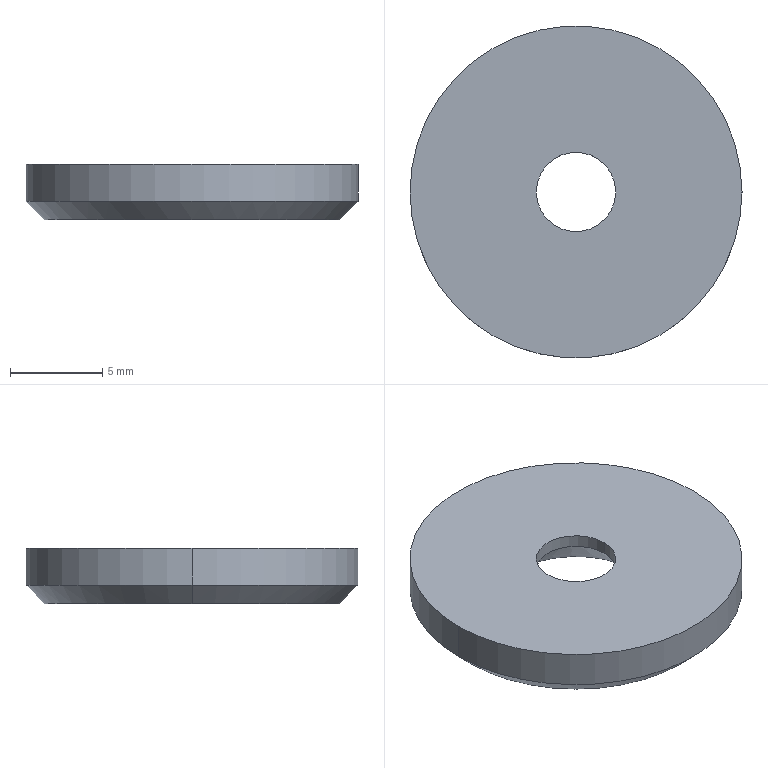Part | STEP file | 14 | 1 solid | 10 faces | box 18 x 18 x 3 mm | volume 644.142 mm3 | cylinder 4 | cone 4 | plane 2 | commonest cylinder face diameters 4.3 x2 18 x2
STEP:
#1=CARTESIAN_POINT('',(0.,0.,0.));
#2=DIRECTION('',(0.,0.,1.));
#3=DIRECTION('',(1.,0.,0.));
#4=AXIS2_PLACEMENT_3D('',#1,#2,#3);
#5=CARTESIAN_POINT('',(-101.,-48.,25.));
#6=VERTEX_POINT('',#5);
#7=CARTESIAN_POINT('',(-119.,-48.,25.));
#8=VERTEX_POINT('',#7);
#9=CARTESIAN_POINT('',(-110.,-48.,25.));
#10=DIRECTION('',(0.,0.,1.));
#11=DIRECTION('',(-1.,0.,0.));
#12=AXIS2_PLACEMENT_3D('',#9,#10,#11);
#13=CIRCLE('',#12,9.);
#14=CARTESIAN_POINT('',(-110.,-48.,23.5));
#15=DIRECTION('',(0.,0.,-1.));
#16=DIRECTION('',(-1.,0.,0.));
#17=AXIS2_PLACEMENT_3D('',#14,#15,#16);
#18=CYLINDRICAL_SURFACE('',#17,9.);
#19=CARTESIAN_POINT('',(6.283,-1.5));
#20=DIRECTION('',(-1.,0.));
#21=VECTOR('',#20,1.);
#22=LINE('',#19,#21);
#23=(GEOMETRIC_REPRESENTATION_CONTEXT(2)PARAMETRIC_REPRESENTATION_CONTEXT()REPRESENTATION_CONTEXT('',''));
#24=DEFINITIONAL_REPRESENTATION('',(#22),#23);
#25=PCURVE('',#18,#24);
#26=CARTESIAN_POINT('',(-105.5,-48.,25.));
#27=DIRECTION('',(0.,0.,1.));
#28=DIRECTION('',(1.,0.,0.));
#29=AXIS2_PLACEMENT_3D('',#26,#27,#28);
#30=PLANE('',#29);
#31=CARTESIAN_POINT('',(-4.5,0.));
#32=DIRECTION('',(-1.,0.));
#33=AXIS2_PLACEMENT_2D('',#31,#32);
#34=CIRCLE('',#33,9.);
#35=(GEOMETRIC_REPRESENTATION_CONTEXT(2)PARAMETRIC_REPRESENTATION_CONTEXT()REPRESENTATION_CONTEXT('',''));
#36=DEFINITIONAL_REPRESENTATION('',(#34),#35);
#37=PCURVE('',#30,#36);
#38=SURFACE_CURVE('',#13,(#25,#37),.PCURVE_S1.);
#39=EDGE_CURVE('',#6,#8,#38,.T.);
#40=ORIENTED_EDGE('',*,*,#39,.F.);
#41=CARTESIAN_POINT('',(-101.,-48.,23.));
#42=VERTEX_POINT('',#41);
#43=CARTESIAN_POINT('',(-101.,-48.,23.5));
#44=DIRECTION('',(0.,0.,-1.));
#45=VECTOR('',#44,1.);
#46=LINE('',#43,#45);
#47=CARTESIAN_POINT('',(3.142,0.));
#48=DIRECTION('',(0.,1.));
#49=VECTOR('',#48,1.);
#50=LINE('',#47,#49);
#51=(GEOMETRIC_REPRESENTATION_CONTEXT(2)PARAMETRIC_REPRESENTATION_CONTEXT()REPRESENTATION_CONTEXT('',''));
#52=DEFINITIONAL_REPRESENTATION('',(#50),#51);
#53=PCURVE('',#18,#52);
#54=CARTESIAN_POINT('',(-110.,-48.,23.5));
#55=DIRECTION('',(0.,0.,-1.));
#56=DIRECTION('',(-1.,0.,0.));
#57=AXIS2_PLACEMENT_3D('',#54,#55,#56);
#58=CYLINDRICAL_SURFACE('',#57,9.);
#59=CARTESIAN_POINT('',(3.142,0.));
#60=DIRECTION('',(0.,1.));
#61=VECTOR('',#60,1.);
#62=LINE('',#59,#61);
#63=(GEOMETRIC_REPRESENTATION_CONTEXT(2)PARAMETRIC_REPRESENTATION_CONTEXT()REPRESENTATION_CONTEXT('',''));
#64=DEFINITIONAL_REPRESENTATION('',(#62),#63);
#65=PCURVE('',#58,#64);
#66=SURFACE_CURVE('',#46,(#53,#65),.PCURVE_S1.);
#67=EDGE_CURVE('',#6,#42,#66,.T.);
#68=ORIENTED_EDGE('',*,*,#67,.T.);
#69=CARTESIAN_POINT('',(-119.,-48.,23.));
#70=VERTEX_POINT('',#69);
#71=CARTESIAN_POINT('',(-110.,-48.,23.));
#72=DIRECTION('',(0.,0.,1.));
#73=DIRECTION('',(-1.,0.,0.));
#74=AXIS2_PLACEMENT_3D('',#71,#72,#73);
#75=CIRCLE('',#74,9.);
#76=CARTESIAN_POINT('',(6.283,0.5));
#77=DIRECTION('',(-1.,0.));
#78=VECTOR('',#77,1.);
#79=LINE('',#76,#78);
#80=(GEOMETRIC_REPRESENTATION_CONTEXT(2)PARAMETRIC_REPRESENTATION_CONTEXT()REPRESENTATION_CONTEXT('',''));
#81=DEFINITIONAL_REPRESENTATION('',(#79),#80);
#82=PCURVE('',#18,#81);
#83=CARTESIAN_POINT('',(-110.,-48.,23.));
#84=DIRECTION('',(0.,0.,1.));
#85=DIRECTION('',(1.,0.,0.));
#86=AXIS2_PLACEMENT_3D('',#83,#84,#85);
#87=CONICAL_SURFACE('',#86,9.,0.7854);
#88=CARTESIAN_POINT('',(-3.142,0.));
#89=DIRECTION('',(1.,0.));
#90=VECTOR('',#89,1.);
#91=LINE('',#88,#90);
#92=(GEOMETRIC_REPRESENTATION_CONTEXT(2)PARAMETRIC_REPRESENTATION_CONTEXT()REPRESENTATION_CONTEXT('',''));
#93=DEFINITIONAL_REPRESENTATION('',(#91),#92);
#94=PCURVE('',#87,#93);
#95=SURFACE_CURVE('',#75,(#82,#94),.PCURVE_S1.);
#96=EDGE_CURVE('',#42,#70,#95,.T.);
#97=ORIENTED_EDGE('',*,*,#96,.T.);
#98=CARTESIAN_POINT('',(-119.,-48.,23.5));
#99=DIRECTION('',(0.,0.,-1.));
#100=VECTOR('',#99,1.);
#101=LINE('',#98,#100);
#102=CARTESIAN_POINT('',(0.,0.));
#103=DIRECTION('',(0.,1.));
#104=VECTOR('',#103,1.);
#105=LINE('',#102,#104);
#106=(GEOMETRIC_REPRESENTATION_CONTEXT(2)PARAMETRIC_REPRESENTATION_CONTEXT()REPRESENTATION_CONTEXT('',''));
#107=DEFINITIONAL_REPRESENTATION('',(#105),#106);
#108=PCURVE('',#18,#107);
#109=CARTESIAN_POINT('',(6.283,0.));
#110=DIRECTION('',(0.,1.));
#111=VECTOR('',#110,1.);
#112=LINE('',#109,#111);
#113=(GEOMETRIC_REPRESENTATION_CONTEXT(2)PARAMETRIC_REPRESENTATION_CONTEXT()REPRESENTATION_CONTEXT('',''));
#114=DEFINITIONAL_REPRESENTATION('',(#112),#113);
#115=PCURVE('',#58,#114);
#116=SURFACE_CURVE('',#101,(#108,#115),.PCURVE_S1.);
#117=EDGE_CURVE('',#8,#70,#116,.T.);
#118=ORIENTED_EDGE('',*,*,#117,.F.);
#119=EDGE_LOOP('',(#40,#68,#97,#118));
#120=FACE_BOUND('',#119,.T.);
#121=ADVANCED_FACE('',(#120),#18,.T.);
#122=CARTESIAN_POINT('',(-112.15,-48.,25.));
#123=VERTEX_POINT('',#122);
#124=CARTESIAN_POINT('',(-112.15,-48.,24.3));
#125=VERTEX_POINT('',#124);
#126=CARTESIAN_POINT('',(-112.15,-48.,24.65));
#127=DIRECTION('',(0.,0.,-1.));
#128=VECTOR('',#127,1.);
#129=LINE('',#126,#128);
#130=CARTESIAN_POINT('',(-110.,-48.,24.65));
#131=DIRECTION('',(0.,0.,-1.));
#132=DIRECTION('',(-1.,0.,0.));
#133=AXIS2_PLACEMENT_3D('',#130,#131,#132);
#134=CYLINDRICAL_SURFACE('',#133,2.15);
#135=CARTESIAN_POINT('',(6.283,0.));
#136=DIRECTION('',(0.,1.));
#137=VECTOR('',#136,1.);
#138=LINE('',#135,#137);
#139=(GEOMETRIC_REPRESENTATION_CONTEXT(2)PARAMETRIC_REPRESENTATION_CONTEXT()REPRESENTATION_CONTEXT('',''));
#140=DEFINITIONAL_REPRESENTATION('',(#138),#139);
#141=PCURVE('',#134,#140);
#142=CARTESIAN_POINT('',(-110.,-48.,24.65));
#143=DIRECTION('',(0.,0.,-1.));
#144=DIRECTION('',(-1.,0.,0.));
#145=AXIS2_PLACEMENT_3D('',#142,#143,#144);
#146=CYLINDRICAL_SURFACE('',#145,2.15);
#147=CARTESIAN_POINT('',(0.,0.));
#148=DIRECTION('',(0.,1.));
#149=VECTOR('',#148,1.);
#150=LINE('',#147,#149);
#151=(GEOMETRIC_REPRESENTATION_CONTEXT(2)PARAMETRIC_REPRESENTATION_CONTEXT()REPRESENTATION_CONTEXT('',''));
#152=DEFINITIONAL_REPRESENTATION('',(#150),#151);
#153=PCURVE('',#146,#152);
#154=SURFACE_CURVE('',#129,(#141,#153),.PCURVE_S1.);
#155=EDGE_CURVE('',#123,#125,#154,.T.);
#156=ORIENTED_EDGE('',*,*,#155,.T.);
#157=CARTESIAN_POINT('',(-107.85,-48.,24.3));
#158=VERTEX_POINT('',#157);
#159=CARTESIAN_POINT('',(-110.,-48.,24.3));
#160=DIRECTION('',(0.,0.,1.));
#161=DIRECTION('',(-1.,0.,0.));
#162=AXIS2_PLACEMENT_3D('',#159,#160,#161);
#163=CIRCLE('',#162,2.15);
#164=CARTESIAN_POINT('',(6.283,0.35));
#165=DIRECTION('',(-1.,0.));
#166=VECTOR('',#165,1.);
#167=LINE('',#164,#166);
#168=(GEOMETRIC_REPRESENTATION_CONTEXT(2)PARAMETRIC_REPRESENTATION_CONTEXT()REPRESENTATION_CONTEXT('',''));
#169=DEFINITIONAL_REPRESENTATION('',(#167),#168);
#170=PCURVE('',#134,#169);
#171=CARTESIAN_POINT('',(-110.,-48.,22.));
#172=DIRECTION('',(0.,0.,-1.));
#173=DIRECTION('',(-1.,0.,0.));
#174=AXIS2_PLACEMENT_3D('',#171,#172,#173);
#175=CONICAL_SURFACE('',#174,4.45,0.7854);
#176=CARTESIAN_POINT('',(6.283,-2.3));
#177=DIRECTION('',(-1.,0.));
#178=VECTOR('',#177,1.);
#179=LINE('',#176,#178);
#180=(GEOMETRIC_REPRESENTATION_CONTEXT(2)PARAMETRIC_REPRESENTATION_CONTEXT()REPRESENTATION_CONTEXT('',''));
#181=DEFINITIONAL_REPRESENTATION('',(#179),#180);
#182=PCURVE('',#175,#181);
#183=SURFACE_CURVE('',#163,(#170,#182),.PCURVE_S1.);
#184=EDGE_CURVE('',#125,#158,#183,.T.);
#185=ORIENTED_EDGE('',*,*,#184,.T.);
#186=CARTESIAN_POINT('',(-107.85,-48.,25.));
#187=VERTEX_POINT('',#186);
#188=CARTESIAN_POINT('',(-107.85,-48.,24.65));
#189=DIRECTION('',(0.,0.,-1.));
#190=VECTOR('',#189,1.);
#191=LINE('',#188,#190);
#192=CARTESIAN_POINT('',(3.142,0.));
#193=DIRECTION('',(0.,1.));
#194=VECTOR('',#193,1.);
#195=LINE('',#192,#194);
#196=(GEOMETRIC_REPRESENTATION_CONTEXT(2)PARAMETRIC_REPRESENTATION_CONTEXT()REPRESENTATION_CONTEXT('',''));
#197=DEFINITIONAL_REPRESENTATION('',(#195),#196);
#198=PCURVE('',#134,#197);
#199=CARTESIAN_POINT('',(3.142,0.));
#200=DIRECTION('',(0.,1.));
#201=VECTOR('',#200,1.);
#202=LINE('',#199,#201);
#203=(GEOMETRIC_REPRESENTATION_CONTEXT(2)PARAMETRIC_REPRESENTATION_CONTEXT()REPRESENTATION_CONTEXT('',''));
#204=DEFINITIONAL_REPRESENTATION('',(#202),#203);
#205=PCURVE('',#146,#204);
#206=SURFACE_CURVE('',#191,(#198,#205),.PCURVE_S1.);
#207=EDGE_CURVE('',#187,#158,#206,.T.);
#208=ORIENTED_EDGE('',*,*,#207,.F.);
#209=CARTESIAN_POINT('',(-110.,-48.,25.));
#210=DIRECTION('',(0.,0.,-1.));
#211=DIRECTION('',(-1.,0.,0.));
#212=AXIS2_PLACEMENT_3D('',#209,#210,#211);
#213=CIRCLE('',#212,2.15);
#214=CARTESIAN_POINT('',(0.,-0.35));
#215=DIRECTION('',(1.,0.));
#216=VECTOR('',#215,1.);
#217=LINE('',#214,#216);
#218=(GEOMETRIC_REPRESENTATION_CONTEXT(2)PARAMETRIC_REPRESENTATION_CONTEXT()REPRESENTATION_CONTEXT('',''));
#219=DEFINITIONAL_REPRESENTATION('',(#217),#218);
#220=PCURVE('',#134,#219);
#221=CARTESIAN_POINT('',(-6.65,0.));
#222=CARTESIAN_POINT('',(-6.65,3.724));
#223=CARTESIAN_POINT('',(-3.425,1.862));
#224=CARTESIAN_POINT('',(-0.2,0.));
#225=CARTESIAN_POINT('',(-3.425,-1.862));
#226=CARTESIAN_POINT('',(-6.65,-3.724));
#227=CARTESIAN_POINT('',(-6.65,0.));
#228=(BOUNDED_CURVE()B_SPLINE_CURVE(2,(#221,#222,#223,#224,#225,#226,#227),.UNSPECIFIED.,.T.,.F.)B_SPLINE_CURVE_WITH_KNOTS((1,2,2,2,2,1),(-2.094,0.,2.094,4.189,6.283,8.378),.UNSPECIFIED.)CURVE()GEOMETRIC_REPRESENTATION_ITEM()RATIONAL_B_SPLINE_CURVE((1.,0.5,1.,0.5,1.,0.5,1.))REPRESENTATION_ITEM(''));
#229=(GEOMETRIC_REPRESENTATION_CONTEXT(2)PARAMETRIC_REPRESENTATION_CONTEXT()REPRESENTATION_CONTEXT('',''));
#230=DEFINITIONAL_REPRESENTATION('',(#228),#229);
#231=PCURVE('',#30,#230);
#232=SURFACE_CURVE('',#213,(#220,#231),.PCURVE_S1.);
#233=EDGE_CURVE('',#187,#123,#232,.T.);
#234=ORIENTED_EDGE('',*,*,#233,.T.);
#235=EDGE_LOOP('',(#156,#185,#208,#234));
#236=FACE_BOUND('',#235,.F.);
#237=ADVANCED_FACE('',(#236),#134,.F.);
#238=CARTESIAN_POINT('',(-102.,-48.,22.));
#239=VERTEX_POINT('',#238);
#240=CARTESIAN_POINT('',(-118.,-48.,22.));
#241=VERTEX_POINT('',#240);
#242=CARTESIAN_POINT('',(-110.,-48.,22.));
#243=DIRECTION('',(0.,0.,1.));
#244=DIRECTION('',(1.,0.,0.));
#245=AXIS2_PLACEMENT_3D('',#242,#243,#244);
#246=CIRCLE('',#245,8.);
#247=CARTESIAN_POINT('',(0.,-1.));
#248=DIRECTION('',(1.,0.));
#249=VECTOR('',#248,1.);
#250=LINE('',#247,#249);
#251=(GEOMETRIC_REPRESENTATION_CONTEXT(2)PARAMETRIC_REPRESENTATION_CONTEXT()REPRESENTATION_CONTEXT('',''));
#252=DEFINITIONAL_REPRESENTATION('',(#250),#251);
#253=PCURVE('',#87,#252);
#254=CARTESIAN_POINT('',(-105.5,-48.,22.));
#255=DIRECTION('',(0.,0.,-1.));
#256=DIRECTION('',(-1.,0.,0.));
#257=AXIS2_PLACEMENT_3D('',#254,#255,#256);
#258=PLANE('',#257);
#259=CARTESIAN_POINT('',(-3.5,0.));
#260=CARTESIAN_POINT('',(-3.5,13.856));
#261=CARTESIAN_POINT('',(8.5,6.928));
#262=CARTESIAN_POINT('',(20.5,0.));
#263=CARTESIAN_POINT('',(8.5,-6.928));
#264=CARTESIAN_POINT('',(-3.5,-13.856));
#265=CARTESIAN_POINT('',(-3.5,0.));
#266=(BOUNDED_CURVE()B_SPLINE_CURVE(2,(#259,#260,#261,#262,#263,#264,#265),.UNSPECIFIED.,.T.,.F.)B_SPLINE_CURVE_WITH_KNOTS((1,2,2,2,2,1),(-2.094,0.,2.094,4.189,6.283,8.378),.UNSPECIFIED.)CURVE()GEOMETRIC_REPRESENTATION_ITEM()RATIONAL_B_SPLINE_CURVE((1.,0.5,1.,0.5,1.,0.5,1.))REPRESENTATION_ITEM(''));
#267=(GEOMETRIC_REPRESENTATION_CONTEXT(2)PARAMETRIC_REPRESENTATION_CONTEXT()REPRESENTATION_CONTEXT('',''));
#268=DEFINITIONAL_REPRESENTATION('',(#266),#267);
#269=PCURVE('',#258,#268);
#270=SURFACE_CURVE('',#246,(#253,#269),.PCURVE_S1.);
#271=EDGE_CURVE('',#239,#241,#270,.T.);
#272=ORIENTED_EDGE('',*,*,#271,.T.);
#273=CARTESIAN_POINT('',(-119.,-48.,23.));
#274=DIRECTION('',(-0.7071,0.,0.7071));
#275=VECTOR('',#274,1.);
#276=LINE('',#273,#275);
#277=CARTESIAN_POINT('',(3.142,0.));
#278=DIRECTION('',(0.,1.));
#279=VECTOR('',#278,1.);
#280=LINE('',#277,#279);
#281=(GEOMETRIC_REPRESENTATION_CONTEXT(2)PARAMETRIC_REPRESENTATION_CONTEXT()REPRESENTATION_CONTEXT('',''));
#282=DEFINITIONAL_REPRESENTATION('',(#280),#281);
#283=PCURVE('',#87,#282);
#284=CARTESIAN_POINT('',(-110.,-48.,23.));
#285=DIRECTION('',(0.,0.,1.));
#286=DIRECTION('',(1.,0.,0.));
#287=AXIS2_PLACEMENT_3D('',#284,#285,#286);
#288=CONICAL_SURFACE('',#287,9.,0.7854);
#289=CARTESIAN_POINT('',(3.142,0.));
#290=DIRECTION('',(0.,1.));
#291=VECTOR('',#290,1.);
#292=LINE('',#289,#291);
#293=(GEOMETRIC_REPRESENTATION_CONTEXT(2)PARAMETRIC_REPRESENTATION_CONTEXT()REPRESENTATION_CONTEXT('',''));
#294=DEFINITIONAL_REPRESENTATION('',(#292),#293);
#295=PCURVE('',#288,#294);
#296=SURFACE_CURVE('',#276,(#283,#295),.PCURVE_S1.);
#297=EDGE_CURVE('',#241,#70,#296,.T.);
#298=ORIENTED_EDGE('',*,*,#297,.T.);
#299=ORIENTED_EDGE('',*,*,#96,.F.);
#300=CARTESIAN_POINT('',(-101.,-48.,23.));
#301=DIRECTION('',(0.7071,0.,0.7071));
#302=VECTOR('',#301,1.);
#303=LINE('',#300,#302);
#304=CARTESIAN_POINT('',(0.,0.));
#305=DIRECTION('',(0.,1.));
#306=VECTOR('',#305,1.);
#307=LINE('',#304,#306);
#308=(GEOMETRIC_REPRESENTATION_CONTEXT(2)PARAMETRIC_REPRESENTATION_CONTEXT()REPRESENTATION_CONTEXT('',''));
#309=DEFINITIONAL_REPRESENTATION('',(#307),#308);
#310=PCURVE('',#87,#309);
#311=CARTESIAN_POINT('',(6.283,0.));
#312=DIRECTION('',(0.,1.));
#313=VECTOR('',#312,1.);
#314=LINE('',#311,#313);
#315=(GEOMETRIC_REPRESENTATION_CONTEXT(2)PARAMETRIC_REPRESENTATION_CONTEXT()REPRESENTATION_CONTEXT('',''));
#316=DEFINITIONAL_REPRESENTATION('',(#314),#315);
#317=PCURVE('',#288,#316);
#318=SURFACE_CURVE('',#303,(#310,#317),.PCURVE_S1.);
#319=EDGE_CURVE('',#239,#42,#318,.T.);
#320=ORIENTED_EDGE('',*,*,#319,.F.);
#321=EDGE_LOOP('',(#272,#298,#299,#320));
#322=FACE_BOUND('',#321,.T.);
#323=ADVANCED_FACE('',(#322),#87,.T.);
#324=CARTESIAN_POINT('',(-114.45,-48.,22.));
#325=VERTEX_POINT('',#324);
#326=CARTESIAN_POINT('',(-114.45,-48.,22.));
#327=DIRECTION('',(-0.7071,0.,-0.7071));
#328=VECTOR('',#327,1.);
#329=LINE('',#326,#328);
#330=CARTESIAN_POINT('',(6.283,0.));
#331=DIRECTION('',(0.,1.));
#332=VECTOR('',#331,1.);
#333=LINE('',#330,#332);
#334=(GEOMETRIC_REPRESENTATION_CONTEXT(2)PARAMETRIC_REPRESENTATION_CONTEXT()REPRESENTATION_CONTEXT('',''));
#335=DEFINITIONAL_REPRESENTATION('',(#333),#334);
#336=PCURVE('',#175,#335);
#337=CARTESIAN_POINT('',(-110.,-48.,22.));
#338=DIRECTION('',(0.,0.,-1.));
#339=DIRECTION('',(-1.,0.,0.));
#340=AXIS2_PLACEMENT_3D('',#337,#338,#339);
#341=CONICAL_SURFACE('',#340,4.45,0.7854);
#342=CARTESIAN_POINT('',(0.,0.));
#343=DIRECTION('',(0.,1.));
#344=VECTOR('',#343,1.);
#345=LINE('',#342,#344);
#346=(GEOMETRIC_REPRESENTATION_CONTEXT(2)PARAMETRIC_REPRESENTATION_CONTEXT()REPRESENTATION_CONTEXT('',''));
#347=DEFINITIONAL_REPRESENTATION('',(#345),#346);
#348=PCURVE('',#341,#347);
#349=SURFACE_CURVE('',#329,(#336,#348),.PCURVE_S1.);
#350=EDGE_CURVE('',#125,#325,#349,.T.);
#351=ORIENTED_EDGE('',*,*,#350,.T.);
#352=CARTESIAN_POINT('',(-105.55,-48.,22.));
#353=VERTEX_POINT('',#352);
#354=CARTESIAN_POINT('',(-110.,-48.,22.));
#355=DIRECTION('',(0.,0.,1.));
#356=DIRECTION('',(-1.,0.,0.));
#357=AXIS2_PLACEMENT_3D('',#354,#355,#356);
#358=CIRCLE('',#357,4.45);
#359=CARTESIAN_POINT('',(6.283,0.));
#360=DIRECTION('',(-1.,0.));
#361=VECTOR('',#360,1.);
#362=LINE('',#359,#361);
#363=(GEOMETRIC_REPRESENTATION_CONTEXT(2)PARAMETRIC_REPRESENTATION_CONTEXT()REPRESENTATION_CONTEXT('',''));
#364=DEFINITIONAL_REPRESENTATION('',(#362),#363);
#365=PCURVE('',#175,#364);
#366=CARTESIAN_POINT('',(8.95,0.));
#367=CARTESIAN_POINT('',(8.95,-7.708));
#368=CARTESIAN_POINT('',(2.275,-3.854));
#369=CARTESIAN_POINT('',(-4.4,0.));
#370=CARTESIAN_POINT('',(2.275,3.854));
#371=CARTESIAN_POINT('',(8.95,7.708));
#372=CARTESIAN_POINT('',(8.95,0.));
#373=(BOUNDED_CURVE()B_SPLINE_CURVE(2,(#366,#367,#368,#369,#370,#371,#372),.UNSPECIFIED.,.T.,.F.)B_SPLINE_CURVE_WITH_KNOTS((1,2,2,2,2,1),(-2.094,0.,2.094,4.189,6.283,8.378),.UNSPECIFIED.)CURVE()GEOMETRIC_REPRESENTATION_ITEM()RATIONAL_B_SPLINE_CURVE((1.,0.5,1.,0.5,1.,0.5,1.))REPRESENTATION_ITEM(''));
#374=(GEOMETRIC_REPRESENTATION_CONTEXT(2)PARAMETRIC_REPRESENTATION_CONTEXT()REPRESENTATION_CONTEXT('',''));
#375=DEFINITIONAL_REPRESENTATION('',(#373),#374);
#376=PCURVE('',#258,#375);
#377=SURFACE_CURVE('',#358,(#365,#376),.PCURVE_S1.);
#378=EDGE_CURVE('',#325,#353,#377,.T.);
#379=ORIENTED_EDGE('',*,*,#378,.T.);
#380=CARTESIAN_POINT('',(-105.55,-48.,22.));
#381=DIRECTION('',(0.7071,0.,-0.7071));
#382=VECTOR('',#381,1.);
#383=LINE('',#380,#382);
#384=CARTESIAN_POINT('',(3.142,0.));
#385=DIRECTION('',(0.,1.));
#386=VECTOR('',#385,1.);
#387=LINE('',#384,#386);
#388=(GEOMETRIC_REPRESENTATION_CONTEXT(2)PARAMETRIC_REPRESENTATION_CONTEXT()REPRESENTATION_CONTEXT('',''));
#389=DEFINITIONAL_REPRESENTATION('',(#387),#388);
#390=PCURVE('',#175,#389);
#391=CARTESIAN_POINT('',(3.142,0.));
#392=DIRECTION('',(0.,1.));
#393=VECTOR('',#392,1.);
#394=LINE('',#391,#393);
#395=(GEOMETRIC_REPRESENTATION_CONTEXT(2)PARAMETRIC_REPRESENTATION_CONTEXT()REPRESENTATION_CONTEXT('',''));
#396=DEFINITIONAL_REPRESENTATION('',(#394),#395);
#397=PCURVE('',#341,#396);
#398=SURFACE_CURVE('',#383,(#390,#397),.PCURVE_S1.);
#399=EDGE_CURVE('',#158,#353,#398,.T.);
#400=ORIENTED_EDGE('',*,*,#399,.F.);
#401=ORIENTED_EDGE('',*,*,#184,.F.);
#402=EDGE_LOOP('',(#351,#379,#400,#401));
#403=FACE_BOUND('',#402,.F.);
#404=ADVANCED_FACE('',(#403),#175,.F.);
#405=CARTESIAN_POINT('',(-110.,-48.,25.));
#406=DIRECTION('',(0.,0.,1.));
#407=DIRECTION('',(-1.,0.,0.));
#408=AXIS2_PLACEMENT_3D('',#405,#406,#407);
#409=CIRCLE('',#408,9.);
#410=CARTESIAN_POINT('',(-4.5,0.));
#411=DIRECTION('',(-1.,0.));
#412=AXIS2_PLACEMENT_2D('',#410,#411);
#413=CIRCLE('',#412,9.);
#414=(GEOMETRIC_REPRESENTATION_CONTEXT(2)PARAMETRIC_REPRESENTATION_CONTEXT()REPRESENTATION_CONTEXT('',''));
#415=DEFINITIONAL_REPRESENTATION('',(#413),#414);
#416=PCURVE('',#30,#415);
#417=CARTESIAN_POINT('',(6.283,-1.5));
#418=DIRECTION('',(-1.,0.));
#419=VECTOR('',#418,1.);
#420=LINE('',#417,#419);
#421=(GEOMETRIC_REPRESENTATION_CONTEXT(2)PARAMETRIC_REPRESENTATION_CONTEXT()REPRESENTATION_CONTEXT('',''));
#422=DEFINITIONAL_REPRESENTATION('',(#420),#421);
#423=PCURVE('',#58,#422);
#424=SURFACE_CURVE('',#409,(#416,#423),.PCURVE_S1.);
#425=EDGE_CURVE('',#8,#6,#424,.T.);
#426=ORIENTED_EDGE('',*,*,#425,.T.);
#427=ORIENTED_EDGE('',*,*,#39,.T.);
#428=EDGE_LOOP('',(#426,#427));
#429=FACE_BOUND('',#428,.T.);
#430=CARTESIAN_POINT('',(-110.,-48.,25.));
#431=DIRECTION('',(0.,0.,-1.));
#432=DIRECTION('',(-1.,0.,0.));
#433=AXIS2_PLACEMENT_3D('',#430,#431,#432);
#434=CIRCLE('',#433,2.15);
#435=CARTESIAN_POINT('',(-6.65,0.));
#436=CARTESIAN_POINT('',(-6.65,3.724));
#437=CARTESIAN_POINT('',(-3.425,1.862));
#438=CARTESIAN_POINT('',(-0.2,0.));
#439=CARTESIAN_POINT('',(-3.425,-1.862));
#440=CARTESIAN_POINT('',(-6.65,-3.724));
#441=CARTESIAN_POINT('',(-6.65,0.));
#442=(BOUNDED_CURVE()B_SPLINE_CURVE(2,(#435,#436,#437,#438,#439,#440,#441),.UNSPECIFIED.,.T.,.F.)B_SPLINE_CURVE_WITH_KNOTS((1,2,2,2,2,1),(-2.094,0.,2.094,4.189,6.283,8.378),.UNSPECIFIED.)CURVE()GEOMETRIC_REPRESENTATION_ITEM()RATIONAL_B_SPLINE_CURVE((1.,0.5,1.,0.5,1.,0.5,1.))REPRESENTATION_ITEM(''));
#443=(GEOMETRIC_REPRESENTATION_CONTEXT(2)PARAMETRIC_REPRESENTATION_CONTEXT()REPRESENTATION_CONTEXT('',''));
#444=DEFINITIONAL_REPRESENTATION('',(#442),#443);
#445=PCURVE('',#30,#444);
#446=CARTESIAN_POINT('',(0.,-0.35));
#447=DIRECTION('',(1.,0.));
#448=VECTOR('',#447,1.);
#449=LINE('',#446,#448);
#450=(GEOMETRIC_REPRESENTATION_CONTEXT(2)PARAMETRIC_REPRESENTATION_CONTEXT()REPRESENTATION_CONTEXT('',''));
#451=DEFINITIONAL_REPRESENTATION('',(#449),#450);
#452=PCURVE('',#146,#451);
#453=SURFACE_CURVE('',#434,(#445,#452),.PCURVE_S1.);
#454=EDGE_CURVE('',#123,#187,#453,.T.);
#455=ORIENTED_EDGE('',*,*,#454,.T.);
#456=ORIENTED_EDGE('',*,*,#233,.T.);
#457=EDGE_LOOP('',(#455,#456));
#458=FACE_BOUND('',#457,.T.);
#459=ADVANCED_FACE('',(#429,#458),#30,.T.);
#460=ORIENTED_EDGE('',*,*,#67,.F.);
#461=ORIENTED_EDGE('',*,*,#425,.F.);
#462=ORIENTED_EDGE('',*,*,#117,.T.);
#463=CARTESIAN_POINT('',(-110.,-48.,23.));
#464=DIRECTION('',(0.,0.,1.));
#465=DIRECTION('',(-1.,0.,0.));
#466=AXIS2_PLACEMENT_3D('',#463,#464,#465);
#467=CIRCLE('',#466,9.);
#468=CARTESIAN_POINT('',(6.283,0.5));
#469=DIRECTION('',(-1.,0.));
#470=VECTOR('',#469,1.);
#471=LINE('',#468,#470);
#472=(GEOMETRIC_REPRESENTATION_CONTEXT(2)PARAMETRIC_REPRESENTATION_CONTEXT()REPRESENTATION_CONTEXT('',''));
#473=DEFINITIONAL_REPRESENTATION('',(#471),#472);
#474=PCURVE('',#58,#473);
#475=CARTESIAN_POINT('',(3.142,0.));
#476=DIRECTION('',(1.,0.));
#477=VECTOR('',#476,1.);
#478=LINE('',#475,#477);
#479=(GEOMETRIC_REPRESENTATION_CONTEXT(2)PARAMETRIC_REPRESENTATION_CONTEXT()REPRESENTATION_CONTEXT('',''));
#480=DEFINITIONAL_REPRESENTATION('',(#478),#479);
#481=PCURVE('',#288,#480);
#482=SURFACE_CURVE('',#467,(#474,#481),.PCURVE_S1.);
#483=EDGE_CURVE('',#70,#42,#482,.T.);
#484=ORIENTED_EDGE('',*,*,#483,.T.);
#485=EDGE_LOOP('',(#460,#461,#462,#484));
#486=FACE_BOUND('',#485,.T.);
#487=ADVANCED_FACE('',(#486),#58,.T.);
#488=CARTESIAN_POINT('',(-110.,-48.,24.3));
#489=DIRECTION('',(0.,0.,1.));
#490=DIRECTION('',(-1.,0.,0.));
#491=AXIS2_PLACEMENT_3D('',#488,#489,#490);
#492=CIRCLE('',#491,2.15);
#493=CARTESIAN_POINT('',(6.283,0.35));
#494=DIRECTION('',(-1.,0.));
#495=VECTOR('',#494,1.);
#496=LINE('',#493,#495);
#497=(GEOMETRIC_REPRESENTATION_CONTEXT(2)PARAMETRIC_REPRESENTATION_CONTEXT()REPRESENTATION_CONTEXT('',''));
#498=DEFINITIONAL_REPRESENTATION('',(#496),#497);
#499=PCURVE('',#146,#498);
#500=CARTESIAN_POINT('',(6.283,-2.3));
#501=DIRECTION('',(-1.,0.));
#502=VECTOR('',#501,1.);
#503=LINE('',#500,#502);
#504=(GEOMETRIC_REPRESENTATION_CONTEXT(2)PARAMETRIC_REPRESENTATION_CONTEXT()REPRESENTATION_CONTEXT('',''));
#505=DEFINITIONAL_REPRESENTATION('',(#503),#504);
#506=PCURVE('',#341,#505);
#507=SURFACE_CURVE('',#492,(#499,#506),.PCURVE_S1.);
#508=EDGE_CURVE('',#158,#125,#507,.T.);
#509=ORIENTED_EDGE('',*,*,#508,.T.);
#510=ORIENTED_EDGE('',*,*,#155,.F.);
#511=ORIENTED_EDGE('',*,*,#454,.T.);
#512=ORIENTED_EDGE('',*,*,#207,.T.);
#513=EDGE_LOOP('',(#509,#510,#511,#512));
#514=FACE_BOUND('',#513,.F.);
#515=ADVANCED_FACE('',(#514),#146,.F.);
#516=ORIENTED_EDGE('',*,*,#297,.F.);
#517=CARTESIAN_POINT('',(-110.,-48.,22.));
#518=DIRECTION('',(0.,0.,1.));
#519=DIRECTION('',(1.,0.,0.));
#520=AXIS2_PLACEMENT_3D('',#517,#518,#519);
#521=CIRCLE('',#520,8.);
#522=CARTESIAN_POINT('',(0.,-1.));
#523=DIRECTION('',(1.,0.));
#524=VECTOR('',#523,1.);
#525=LINE('',#522,#524);
#526=(GEOMETRIC_REPRESENTATION_CONTEXT(2)PARAMETRIC_REPRESENTATION_CONTEXT()REPRESENTATION_CONTEXT('',''));
#527=DEFINITIONAL_REPRESENTATION('',(#525),#526);
#528=PCURVE('',#288,#527);
#529=CARTESIAN_POINT('',(-3.5,0.));
#530=CARTESIAN_POINT('',(-3.5,13.856));
#531=CARTESIAN_POINT('',(8.5,6.928));
#532=CARTESIAN_POINT('',(20.5,0.));
#533=CARTESIAN_POINT('',(8.5,-6.928));
#534=CARTESIAN_POINT('',(-3.5,-13.856));
#535=CARTESIAN_POINT('',(-3.5,0.));
#536=(BOUNDED_CURVE()B_SPLINE_CURVE(2,(#529,#530,#531,#532,#533,#534,#535),.UNSPECIFIED.,.T.,.F.)B_SPLINE_CURVE_WITH_KNOTS((1,2,2,2,2,1),(-2.094,0.,2.094,4.189,6.283,8.378),.UNSPECIFIED.)CURVE()GEOMETRIC_REPRESENTATION_ITEM()RATIONAL_B_SPLINE_CURVE((1.,0.5,1.,0.5,1.,0.5,1.))REPRESENTATION_ITEM(''));
#537=(GEOMETRIC_REPRESENTATION_CONTEXT(2)PARAMETRIC_REPRESENTATION_CONTEXT()REPRESENTATION_CONTEXT('',''));
#538=DEFINITIONAL_REPRESENTATION('',(#536),#537);
#539=PCURVE('',#258,#538);
#540=SURFACE_CURVE('',#521,(#528,#539),.PCURVE_S1.);
#541=EDGE_CURVE('',#241,#239,#540,.T.);
#542=ORIENTED_EDGE('',*,*,#541,.T.);
#543=ORIENTED_EDGE('',*,*,#319,.T.);
#544=ORIENTED_EDGE('',*,*,#483,.F.);
#545=EDGE_LOOP('',(#516,#542,#543,#544));
#546=FACE_BOUND('',#545,.T.);
#547=ADVANCED_FACE('',(#546),#288,.T.);
#548=CARTESIAN_POINT('',(-110.,-48.,22.));
#549=DIRECTION('',(0.,0.,1.));
#550=DIRECTION('',(-1.,0.,0.));
#551=AXIS2_PLACEMENT_3D('',#548,#549,#550);
#552=CIRCLE('',#551,4.45);
#553=CARTESIAN_POINT('',(6.283,0.));
#554=DIRECTION('',(-1.,0.));
#555=VECTOR('',#554,1.);
#556=LINE('',#553,#555);
#557=(GEOMETRIC_REPRESENTATION_CONTEXT(2)PARAMETRIC_REPRESENTATION_CONTEXT()REPRESENTATION_CONTEXT('',''));
#558=DEFINITIONAL_REPRESENTATION('',(#556),#557);
#559=PCURVE('',#341,#558);
#560=CARTESIAN_POINT('',(8.95,0.));
#561=CARTESIAN_POINT('',(8.95,-7.708));
#562=CARTESIAN_POINT('',(2.275,-3.854));
#563=CARTESIAN_POINT('',(-4.4,0.));
#564=CARTESIAN_POINT('',(2.275,3.854));
#565=CARTESIAN_POINT('',(8.95,7.708));
#566=CARTESIAN_POINT('',(8.95,0.));
#567=(BOUNDED_CURVE()B_SPLINE_CURVE(2,(#560,#561,#562,#563,#564,#565,#566),.UNSPECIFIED.,.T.,.F.)B_SPLINE_CURVE_WITH_KNOTS((1,2,2,2,2,1),(-2.094,0.,2.094,4.189,6.283,8.378),.UNSPECIFIED.)CURVE()GEOMETRIC_REPRESENTATION_ITEM()RATIONAL_B_SPLINE_CURVE((1.,0.5,1.,0.5,1.,0.5,1.))REPRESENTATION_ITEM(''));
#568=(GEOMETRIC_REPRESENTATION_CONTEXT(2)PARAMETRIC_REPRESENTATION_CONTEXT()REPRESENTATION_CONTEXT('',''));
#569=DEFINITIONAL_REPRESENTATION('',(#567),#568);
#570=PCURVE('',#258,#569);
#571=SURFACE_CURVE('',#552,(#559,#570),.PCURVE_S1.);
#572=EDGE_CURVE('',#353,#325,#571,.T.);
#573=ORIENTED_EDGE('',*,*,#572,.T.);
#574=ORIENTED_EDGE('',*,*,#350,.F.);
#575=ORIENTED_EDGE('',*,*,#508,.F.);
#576=ORIENTED_EDGE('',*,*,#399,.T.);
#577=EDGE_LOOP('',(#573,#574,#575,#576));
#578=FACE_BOUND('',#577,.F.);
#579=ADVANCED_FACE('',(#578),#341,.F.);
#580=ORIENTED_EDGE('',*,*,#271,.F.);
#581=ORIENTED_EDGE('',*,*,#541,.F.);
#582=EDGE_LOOP('',(#580,#581));
#583=FACE_BOUND('',#582,.T.);
#584=ORIENTED_EDGE('',*,*,#378,.T.);
#585=ORIENTED_EDGE('',*,*,#572,.T.);
#586=EDGE_LOOP('',(#584,#585));
#587=FACE_BOUND('',#586,.T.);
#588=ADVANCED_FACE('',(#583,#587),#258,.T.);
#589=CLOSED_SHELL('',(#121,#237,#323,#404,#459,#487,#515,#547,#579,#588));
#590=MANIFOLD_SOLID_BREP('',#589);
#591=(LENGTH_UNIT()NAMED_UNIT(*)SI_UNIT(.MILLI.,.METRE.));
#592=UNCERTAINTY_MEASURE_WITH_UNIT(LENGTH_MEASURE(0.0000001),#591,'','');
#593=(NAMED_UNIT(*)PLANE_ANGLE_UNIT()SI_UNIT($,.RADIAN.));
#594=(NAMED_UNIT(*)SI_UNIT($,.STERADIAN.)SOLID_ANGLE_UNIT());
#595=(GEOMETRIC_REPRESENTATION_CONTEXT(3)GLOBAL_UNCERTAINTY_ASSIGNED_CONTEXT((#592))GLOBAL_UNIT_ASSIGNED_CONTEXT((#591,#593,#594))REPRESENTATION_CONTEXT('',''));
#596=ADVANCED_BREP_SHAPE_REPRESENTATION('',(#4,#590),#595);